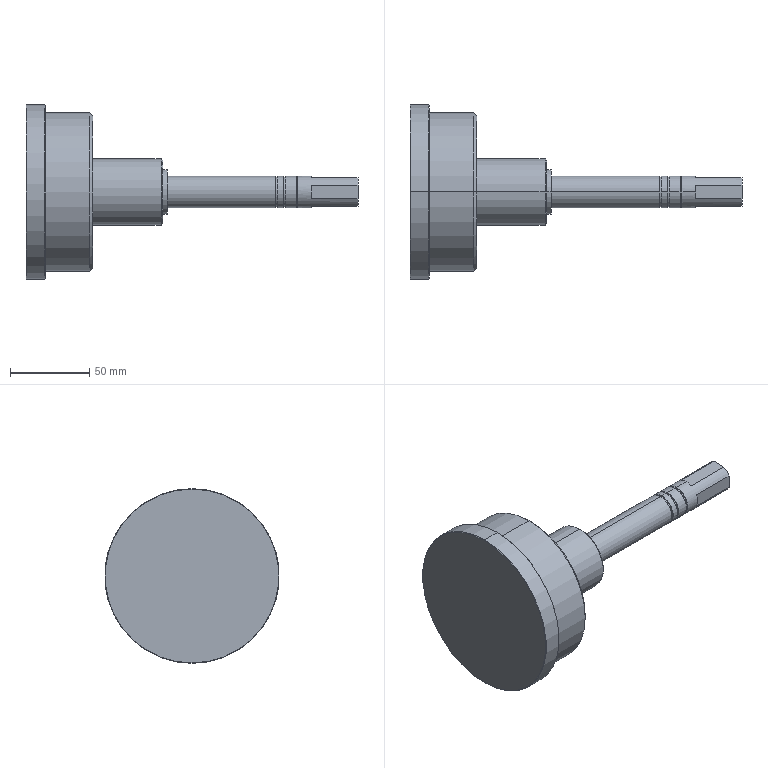Part | STEP file | film pull movable wheel_SUS304 | 1 solid | 50 faces | box 209 x 110 x 110 mm | volume 448642 mm3 | cylinder 22 | plane 20 | cone 8 | commonest cylinder face diameters 20 x8 18.85 x6 28 x2 42 x2 100 x2 110 x2